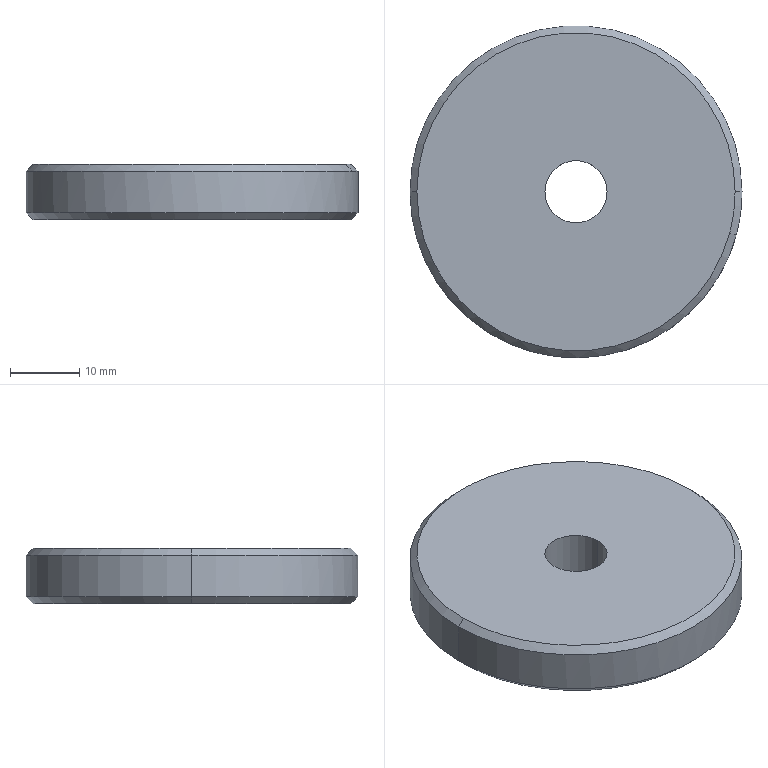Part | CATIA | 1 solid | 12 faces | box 48 x 48 x 8 mm | volume 13819 mm3 | cone 6 | cylinder 4 | plane 2 | commonest cylinder face diameters 9 x2 48 x2
STEP:
#1=CARTESIAN_POINT('',(-494.5,250.,-217.));
#2=VERTEX_POINT('',#1);
#3=CARTESIAN_POINT('',(-494.5,250.,-225.));
#4=VERTEX_POINT('',#3);
#5=CARTESIAN_POINT('',(-494.5,250.,-221.));
#6=DIRECTION('',(0.,0.,1.));
#7=VECTOR('',#6,1.);
#8=LINE('',#5,#7);
#9=EDGE_CURVE('',#2,#4,#8,.F.);
#10=ORIENTED_EDGE('',*,*,#9,.F.);
#11=CARTESIAN_POINT('',(-485.5,250.,-217.));
#12=VERTEX_POINT('',#11);
#13=CARTESIAN_POINT('',(-490.,250.,-217.));
#14=DIRECTION('',(0.,0.,1.));
#15=AXIS2_PLACEMENT_3D('',#13,#14,$);
#16=CIRCLE('',#15,4.5);
#17=EDGE_CURVE('',#2,#12,#16,.T.);
#18=ORIENTED_EDGE('',*,*,#17,.T.);
#19=CARTESIAN_POINT('',(-485.5,250.,-225.));
#20=VERTEX_POINT('',#19);
#21=CARTESIAN_POINT('',(-485.5,250.,-221.));
#22=DIRECTION('',(0.,0.,1.));
#23=VECTOR('',#22,1.);
#24=LINE('',#21,#23);
#25=EDGE_CURVE('',#12,#20,#24,.F.);
#26=ORIENTED_EDGE('',*,*,#25,.T.);
#27=CARTESIAN_POINT('',(-490.,250.,-225.));
#28=DIRECTION('',(0.,0.,1.));
#29=AXIS2_PLACEMENT_3D('',#27,#28,$);
#30=CIRCLE('',#29,4.5);
#31=EDGE_CURVE('',#4,#20,#30,.T.);
#32=ORIENTED_EDGE('',*,*,#31,.F.);
#33=EDGE_LOOP('',(#10,#18,#26,#32));
#34=FACE_OUTER_BOUND('',#33,.T.);
#35=CARTESIAN_POINT('',(-490.,250.,-221.));
#36=DIRECTION('',(0.,0.,1.));
#37=DIRECTION('',(-1.,0.,0.));
#38=AXIS2_PLACEMENT_3D('',#35,#36,#37);
#39=CYLINDRICAL_SURFACE('',#38,4.5);
#40=ADVANCED_FACE('',(#34),#39,.F.);
#41=ORIENTED_EDGE('',*,*,#25,.F.);
#42=CARTESIAN_POINT('',(-490.,250.,-217.));
#43=DIRECTION('',(0.,0.,1.));
#44=AXIS2_PLACEMENT_3D('',#42,#43,$);
#45=CIRCLE('',#44,4.5);
#46=EDGE_CURVE('',#12,#2,#45,.T.);
#47=ORIENTED_EDGE('',*,*,#46,.T.);
#48=ORIENTED_EDGE('',*,*,#9,.T.);
#49=CARTESIAN_POINT('',(-490.,250.,-225.));
#50=DIRECTION('',(0.,0.,1.));
#51=AXIS2_PLACEMENT_3D('',#49,#50,$);
#52=CIRCLE('',#51,4.5);
#53=EDGE_CURVE('',#20,#4,#52,.T.);
#54=ORIENTED_EDGE('',*,*,#53,.F.);
#55=EDGE_LOOP('',(#41,#47,#48,#54));
#56=FACE_OUTER_BOUND('',#55,.T.);
#57=CARTESIAN_POINT('',(-490.,250.,-221.));
#58=DIRECTION('',(0.,0.,1.));
#59=DIRECTION('',(1.,0.,0.));
#60=AXIS2_PLACEMENT_3D('',#57,#58,#59);
#61=CYLINDRICAL_SURFACE('',#60,4.5);
#62=ADVANCED_FACE('',(#56),#61,.F.);
#63=CARTESIAN_POINT('',(-513.,250.,-217.));
#64=VERTEX_POINT('',#63);
#65=CARTESIAN_POINT('',(-467.791,244.02,-217.));
#66=VERTEX_POINT('',#65);
#67=CARTESIAN_POINT('',(-490.,250.,-217.));
#68=DIRECTION('',(0.,0.,1.));
#69=AXIS2_PLACEMENT_3D('',#67,#68,$);
#70=CIRCLE('',#69,23.);
#71=EDGE_CURVE('',#64,#66,#70,.T.);
#72=ORIENTED_EDGE('',*,*,#71,.T.);
#73=CARTESIAN_POINT('',(-467.,250.,-217.));
#74=VERTEX_POINT('',#73);
#75=CARTESIAN_POINT('',(-490.,250.,-217.));
#76=DIRECTION('',(0.,0.,1.));
#77=AXIS2_PLACEMENT_3D('',#75,#76,$);
#78=CIRCLE('',#77,23.);
#79=EDGE_CURVE('',#66,#74,#78,.T.);
#80=ORIENTED_EDGE('',*,*,#79,.T.);
#81=CARTESIAN_POINT('',(-490.,250.,-217.));
#82=DIRECTION('',(0.,0.,1.));
#83=AXIS2_PLACEMENT_3D('',#81,#82,$);
#84=CIRCLE('',#83,23.);
#85=EDGE_CURVE('',#74,#64,#84,.T.);
#86=ORIENTED_EDGE('',*,*,#85,.T.);
#87=EDGE_LOOP('',(#72,#80,#86));
#88=FACE_OUTER_BOUND('',#87,.T.);
#89=ORIENTED_EDGE('',*,*,#17,.F.);
#90=ORIENTED_EDGE('',*,*,#46,.F.);
#91=EDGE_LOOP('',(#89,#90));
#92=FACE_BOUND('',#91,.T.);
#93=CARTESIAN_POINT('',(0.,0.,-217.));
#94=DIRECTION('',(0.,0.,1.));
#95=DIRECTION('',(1.,0.,0.));
#96=AXIS2_PLACEMENT_3D('',#93,#94,#95);
#97=PLANE('',#96);
#98=ADVANCED_FACE('',(#88,#92),#97,.T.);
#99=CARTESIAN_POINT('',(-467.,250.,-225.));
#100=VERTEX_POINT('',#99);
#101=CARTESIAN_POINT('',(-513.,250.,-225.));
#102=VERTEX_POINT('',#101);
#103=CARTESIAN_POINT('',(-490.,250.,-225.));
#104=DIRECTION('',(0.,0.,1.));
#105=AXIS2_PLACEMENT_3D('',#103,#104,$);
#106=CIRCLE('',#105,23.);
#107=EDGE_CURVE('',#100,#102,#106,.T.);
#108=ORIENTED_EDGE('',*,*,#107,.F.);
#109=CARTESIAN_POINT('',(-468.471,241.907,-225.));
#110=VERTEX_POINT('',#109);
#111=CARTESIAN_POINT('',(-490.,250.,-225.));
#112=DIRECTION('',(0.,0.,1.));
#113=AXIS2_PLACEMENT_3D('',#111,#112,$);
#114=CIRCLE('',#113,23.);
#115=EDGE_CURVE('',#110,#100,#114,.T.);
#116=ORIENTED_EDGE('',*,*,#115,.F.);
#117=CARTESIAN_POINT('',(-490.,250.,-225.));
#118=DIRECTION('',(0.,0.,1.));
#119=AXIS2_PLACEMENT_3D('',#117,#118,$);
#120=CIRCLE('',#119,23.);
#121=EDGE_CURVE('',#102,#110,#120,.T.);
#122=ORIENTED_EDGE('',*,*,#121,.F.);
#123=EDGE_LOOP('',(#108,#116,#122));
#124=FACE_OUTER_BOUND('',#123,.T.);
#125=ORIENTED_EDGE('',*,*,#53,.T.);
#126=ORIENTED_EDGE('',*,*,#31,.T.);
#127=EDGE_LOOP('',(#125,#126));
#128=FACE_BOUND('',#127,.T.);
#129=CARTESIAN_POINT('',(0.,0.,-225.));
#130=DIRECTION('',(0.,0.,1.));
#131=DIRECTION('',(1.,0.,0.));
#132=AXIS2_PLACEMENT_3D('',#129,#130,#131);
#133=PLANE('',#132);
#134=ADVANCED_FACE('',(#124,#128),#133,.F.);
#135=CARTESIAN_POINT('',(-466.825,243.76,-218.));
#136=VERTEX_POINT('',#135);
#137=CARTESIAN_POINT('',(340902.764,-91679.216,-353747.391));
#138=DIRECTION('',(0.6828,-0.1839,-0.7071));
#139=VECTOR('',#138,1.);
#140=LINE('',#137,#139);
#141=EDGE_CURVE('',#66,#136,#140,.T.);
#142=ORIENTED_EDGE('',*,*,#141,.F.);
#143=ORIENTED_EDGE('',*,*,#71,.F.);
#144=CARTESIAN_POINT('',(-514.,250.,-218.));
#145=VERTEX_POINT('',#144);
#146=CARTESIAN_POINT('',(-354043.391,250.003,-353747.391));
#147=DIRECTION('',(-0.7071,0.000000006,-0.7071));
#148=VECTOR('',#147,1.);
#149=LINE('',#146,#148);
#150=EDGE_CURVE('',#64,#145,#149,.T.);
#151=ORIENTED_EDGE('',*,*,#150,.T.);
#152=CARTESIAN_POINT('',(-490.,250.,-218.));
#153=DIRECTION('',(0.,0.,-1.));
#154=AXIS2_PLACEMENT_3D('',#152,#153,$);
#155=CIRCLE('',#154,24.);
#156=EDGE_CURVE('',#145,#136,#155,.F.);
#157=ORIENTED_EDGE('',*,*,#156,.T.);
#158=EDGE_LOOP('',(#142,#143,#151,#157));
#159=FACE_OUTER_BOUND('',#158,.T.);
#160=CARTESIAN_POINT('',(-490.,250.,-194.));
#161=DIRECTION('',(0.,0.,-1.));
#162=DIRECTION('',(0.9656,-0.26,0.));
#163=AXIS2_PLACEMENT_3D('',#160,#161,#162);
#164=CONICAL_SURFACE('',#163,0.,0.7854);
#165=ADVANCED_FACE('',(#159),#164,.T.);
#166=ORIENTED_EDGE('',*,*,#141,.T.);
#167=CARTESIAN_POINT('',(-466.,250.,-218.));
#168=VERTEX_POINT('',#167);
#169=CARTESIAN_POINT('',(-490.,250.,-218.));
#170=DIRECTION('',(0.,0.,-1.));
#171=AXIS2_PLACEMENT_3D('',#169,#170,$);
#172=CIRCLE('',#171,24.);
#173=EDGE_CURVE('',#136,#168,#172,.F.);
#174=ORIENTED_EDGE('',*,*,#173,.T.);
#175=CARTESIAN_POINT('',(353063.391,250.,-353747.391));
#176=DIRECTION('',(0.7071,0.,-0.7071));
#177=VECTOR('',#176,1.);
#178=LINE('',#175,#177);
#179=EDGE_CURVE('',#74,#168,#178,.T.);
#180=ORIENTED_EDGE('',*,*,#179,.F.);
#181=ORIENTED_EDGE('',*,*,#79,.F.);
#182=EDGE_LOOP('',(#166,#174,#180,#181));
#183=FACE_OUTER_BOUND('',#182,.T.);
#184=CARTESIAN_POINT('',(-490.,250.,-194.));
#185=DIRECTION('',(0.,0.,-1.));
#186=DIRECTION('',(-0.9656,0.26,0.));
#187=AXIS2_PLACEMENT_3D('',#184,#185,#186);
#188=CONICAL_SURFACE('',#187,0.,0.7854);
#189=ADVANCED_FACE('',(#183),#188,.T.);
#190=ORIENTED_EDGE('',*,*,#179,.T.);
#191=CARTESIAN_POINT('',(-490.,250.,-218.));
#192=DIRECTION('',(0.,0.,-1.));
#193=AXIS2_PLACEMENT_3D('',#191,#192,$);
#194=CIRCLE('',#193,24.);
#195=EDGE_CURVE('',#168,#145,#194,.F.);
#196=ORIENTED_EDGE('',*,*,#195,.T.);
#197=ORIENTED_EDGE('',*,*,#150,.F.);
#198=ORIENTED_EDGE('',*,*,#85,.F.);
#199=EDGE_LOOP('',(#190,#196,#197,#198));
#200=FACE_OUTER_BOUND('',#199,.T.);
#201=CARTESIAN_POINT('',(-490.,250.,-194.));
#202=DIRECTION('',(0.,0.,-1.));
#203=DIRECTION('',(-1.,0.,0.));
#204=AXIS2_PLACEMENT_3D('',#201,#202,#203);
#205=CONICAL_SURFACE('',#204,0.,0.7854);
#206=ADVANCED_FACE('',(#200),#205,.T.);
#207=CARTESIAN_POINT('',(-466.,250.,-224.));
#208=VERTEX_POINT('',#207);
#209=CARTESIAN_POINT('',(353063.391,250.,353305.391));
#210=DIRECTION('',(0.7071,0.,0.7071));
#211=VECTOR('',#210,1.);
#212=LINE('',#209,#211);
#213=EDGE_CURVE('',#208,#100,#212,.F.);
#214=ORIENTED_EDGE('',*,*,#213,.T.);
#215=ORIENTED_EDGE('',*,*,#107,.T.);
#216=CARTESIAN_POINT('',(-514.,250.,-224.));
#217=VERTEX_POINT('',#216);
#218=CARTESIAN_POINT('',(-354043.391,250.,353305.391));
#219=DIRECTION('',(-0.7071,0.,0.7071));
#220=VECTOR('',#219,1.);
#221=LINE('',#218,#220);
#222=EDGE_CURVE('',#217,#102,#221,.F.);
#223=ORIENTED_EDGE('',*,*,#222,.F.);
#224=CARTESIAN_POINT('',(-490.,250.,-224.));
#225=DIRECTION('',(0.,0.,1.));
#226=AXIS2_PLACEMENT_3D('',#224,#225,$);
#227=CIRCLE('',#226,24.);
#228=EDGE_CURVE('',#208,#217,#227,.T.);
#229=ORIENTED_EDGE('',*,*,#228,.F.);
#230=EDGE_LOOP('',(#214,#215,#223,#229));
#231=FACE_OUTER_BOUND('',#230,.T.);
#232=CARTESIAN_POINT('',(-490.,250.,-248.));
#233=DIRECTION('',(0.,0.,1.));
#234=DIRECTION('',(1.,0.,0.));
#235=AXIS2_PLACEMENT_3D('',#232,#233,#234);
#236=CONICAL_SURFACE('',#235,0.,0.7854);
#237=ADVANCED_FACE('',(#231),#236,.T.);
#238=CARTESIAN_POINT('',(-467.535,241.555,-224.));
#239=VERTEX_POINT('',#238);
#240=CARTESIAN_POINT('',(330454.3,-124152.051,353305.391));
#241=DIRECTION('',(0.6619,-0.2488,0.7071));
#242=VECTOR('',#241,1.);
#243=LINE('',#240,#242);
#244=EDGE_CURVE('',#110,#239,#243,.T.);
#245=ORIENTED_EDGE('',*,*,#244,.F.);
#246=ORIENTED_EDGE('',*,*,#115,.T.);
#247=ORIENTED_EDGE('',*,*,#213,.F.);
#248=CARTESIAN_POINT('',(-490.,250.,-224.));
#249=DIRECTION('',(0.,0.,1.));
#250=AXIS2_PLACEMENT_3D('',#248,#249,$);
#251=CIRCLE('',#250,24.);
#252=EDGE_CURVE('',#239,#208,#251,.T.);
#253=ORIENTED_EDGE('',*,*,#252,.F.);
#254=EDGE_LOOP('',(#245,#246,#247,#253));
#255=FACE_OUTER_BOUND('',#254,.T.);
#256=CARTESIAN_POINT('',(-490.,250.,-248.));
#257=DIRECTION('',(0.,0.,1.));
#258=DIRECTION('',(0.9361,-0.3519,0.));
#259=AXIS2_PLACEMENT_3D('',#256,#257,#258);
#260=CONICAL_SURFACE('',#259,0.,0.7854);
#261=ADVANCED_FACE('',(#255),#260,.T.);
#262=ORIENTED_EDGE('',*,*,#244,.T.);
#263=CARTESIAN_POINT('',(-490.,250.,-224.));
#264=DIRECTION('',(0.,0.,1.));
#265=AXIS2_PLACEMENT_3D('',#263,#264,$);
#266=CIRCLE('',#265,24.);
#267=EDGE_CURVE('',#217,#239,#266,.T.);
#268=ORIENTED_EDGE('',*,*,#267,.F.);
#269=ORIENTED_EDGE('',*,*,#222,.T.);
#270=ORIENTED_EDGE('',*,*,#121,.T.);
#271=EDGE_LOOP('',(#262,#268,#269,#270));
#272=FACE_OUTER_BOUND('',#271,.T.);
#273=CARTESIAN_POINT('',(-490.,250.,-248.));
#274=DIRECTION('',(0.,0.,1.));
#275=DIRECTION('',(-0.9361,0.3519,0.));
#276=AXIS2_PLACEMENT_3D('',#273,#274,#275);
#277=CONICAL_SURFACE('',#276,0.,0.7854);
#278=ADVANCED_FACE('',(#272),#277,.T.);
#279=CARTESIAN_POINT('',(-466.,250.,-221.));
#280=DIRECTION('',(0.,0.,1.));
#281=VECTOR('',#280,1.);
#282=LINE('',#279,#281);
#283=EDGE_CURVE('',#168,#208,#282,.F.);
#284=ORIENTED_EDGE('',*,*,#283,.F.);
#285=ORIENTED_EDGE('',*,*,#173,.F.);
#286=ORIENTED_EDGE('',*,*,#156,.F.);
#287=CARTESIAN_POINT('',(-514.,250.,-221.));
#288=DIRECTION('',(0.,0.,1.));
#289=VECTOR('',#288,1.);
#290=LINE('',#287,#289);
#291=EDGE_CURVE('',#145,#217,#290,.F.);
#292=ORIENTED_EDGE('',*,*,#291,.T.);
#293=ORIENTED_EDGE('',*,*,#267,.T.);
#294=ORIENTED_EDGE('',*,*,#252,.T.);
#295=EDGE_LOOP('',(#284,#285,#286,#292,#293,#294));
#296=FACE_OUTER_BOUND('',#295,.T.);
#297=CARTESIAN_POINT('',(-490.,250.,-221.));
#298=DIRECTION('',(0.,0.,1.));
#299=DIRECTION('',(-1.,0.,0.));
#300=AXIS2_PLACEMENT_3D('',#297,#298,#299);
#301=CYLINDRICAL_SURFACE('',#300,24.);
#302=ADVANCED_FACE('',(#296),#301,.T.);
#303=ORIENTED_EDGE('',*,*,#291,.F.);
#304=ORIENTED_EDGE('',*,*,#195,.F.);
#305=ORIENTED_EDGE('',*,*,#283,.T.);
#306=ORIENTED_EDGE('',*,*,#228,.T.);
#307=EDGE_LOOP('',(#303,#304,#305,#306));
#308=FACE_OUTER_BOUND('',#307,.T.);
#309=CARTESIAN_POINT('',(-490.,250.,-221.));
#310=DIRECTION('',(0.,0.,1.));
#311=DIRECTION('',(1.,0.,0.));
#312=AXIS2_PLACEMENT_3D('',#309,#310,#311);
#313=CYLINDRICAL_SURFACE('',#312,24.);
#314=ADVANCED_FACE('',(#308),#313,.T.);
#315=CLOSED_SHELL('',(#40,#62,#98,#134,#165,#189,#206,#237,#261,#278,#302,#314));
#316=MANIFOLD_SOLID_BREP('',#315);
#317=(LENGTH_UNIT()NAMED_UNIT(*)SI_UNIT(.MILLI.,.METRE.));
#318=UNCERTAINTY_MEASURE_WITH_UNIT(LENGTH_MEASURE(0.005),#317,'','');
#319=(NAMED_UNIT(*)PLANE_ANGLE_UNIT()SI_UNIT($,.RADIAN.));
#320=(NAMED_UNIT(*)SI_UNIT($,.STERADIAN.)SOLID_ANGLE_UNIT());
#321=(GEOMETRIC_REPRESENTATION_CONTEXT(3)GLOBAL_UNCERTAINTY_ASSIGNED_CONTEXT((#318))GLOBAL_UNIT_ASSIGNED_CONTEXT((#317,#319,#320))REPRESENTATION_CONTEXT('',''));
#322=ADVANCED_BREP_SHAPE_REPRESENTATION('',(#316),#321);